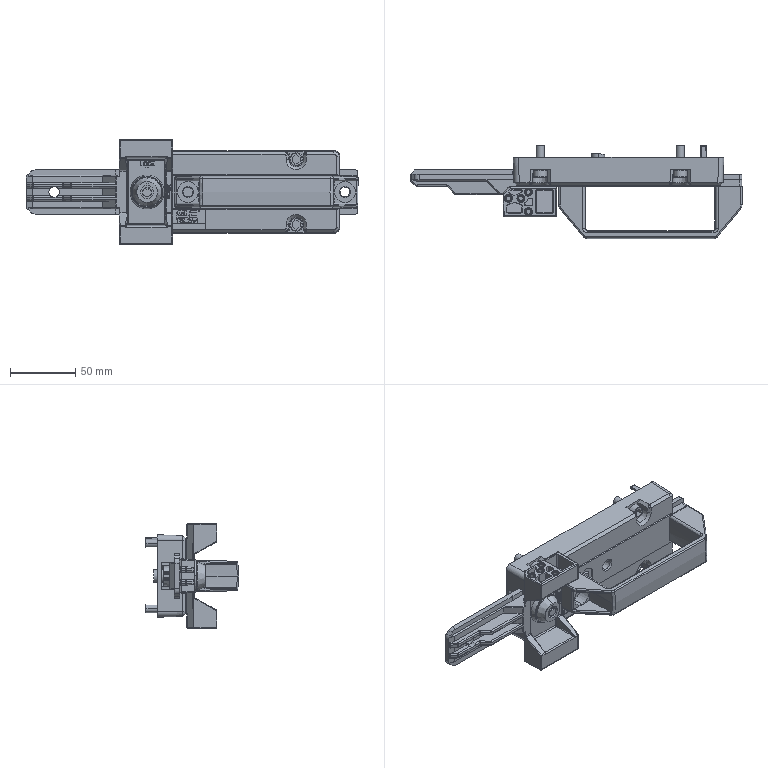Part | SolidWorks | features BaseBody 17, ICE 1 | 17 solids | 4989 faces | volume 237710 mm3 | plane 3035 | cylinder 1415 | spline 330 | cone 127 | torus 56 | sphere 26 | commonest cylinder face diameters 6 x970 2 x143 1 x93 6.5 x56 4 x28 10 x23